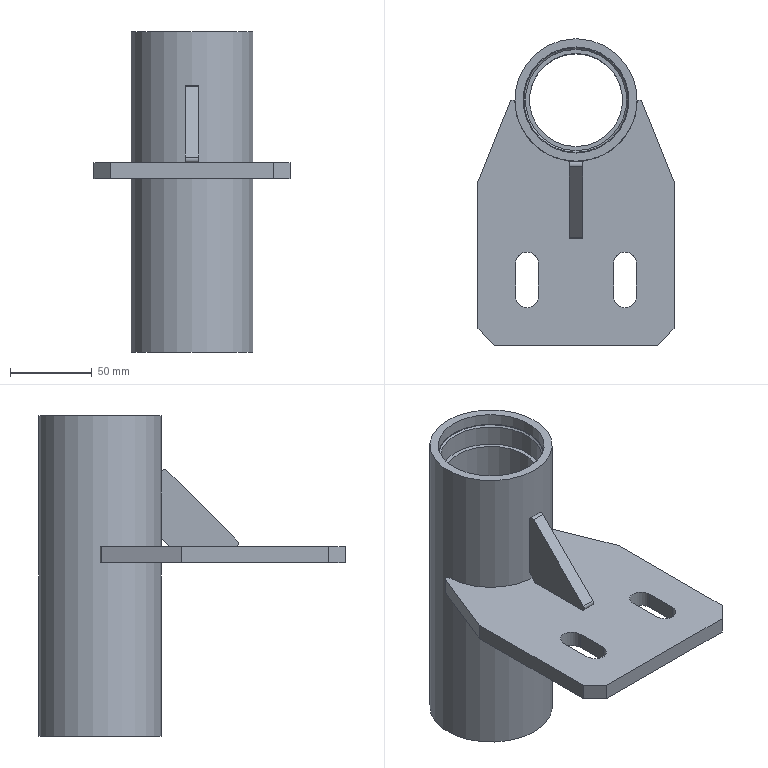Part | STEP file | HL4GZ-1.313.026 (steering rod mounting seat) | 3 solids | 46 faces | box 120.001 x 187.5 x 196 mm | volume 489671 mm3 | plane 27 | cylinder 17 | cone 2 | commonest cylinder face diameters 2 x4 14 x4 4 x2 62 x2 65 x2 75 x2